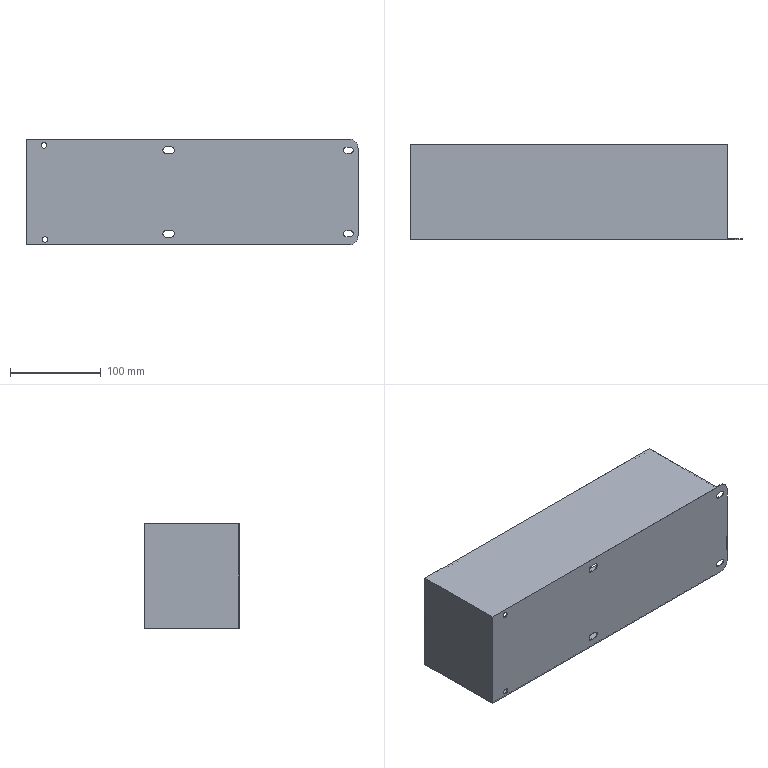Part | SolidWorks | features MoveFace 16, ICE 8, Fillet 2, Extrusion 1, HoleWzd 1, Scale 1, Shell 1 | 1 solid | 68 faces | box 366 x 105 x 116.75 mm | volume 129942 mm3 | plane 38 | cylinder 30 | commonest cylinder face diameters 4.95 x8 15 x8 6 x4 6.4 x4 7.505 x2 7.743 x2